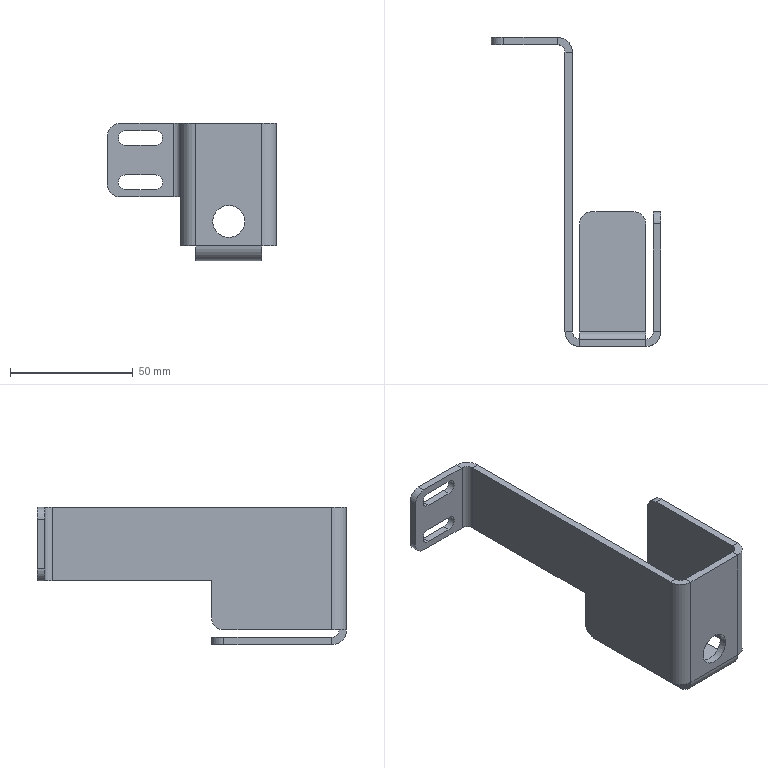Part | NX | features BREP 1 | 1 solid | 55 faces | box 69 x 126 x 56 mm | volume 33216 mm3 | plane 35 | cylinder 20 | commonest cylinder face diameters 6 x8 10 x7 12 x4 13 x1
STEP:
#1=CARTESIAN_POINT('',(0.,117.,30.));
#2=VERTEX_POINT('',#1);
#3=CARTESIAN_POINT('',(-3.,117.,30.));
#4=VERTEX_POINT('',#3);
#5=CARTESIAN_POINT('',(0.,117.,30.));
#6=DIRECTION('',(-1.,0.,0.));
#7=VECTOR('',#6,1000.);
#8=LINE('',#5,#7);
#9=EDGE_CURVE('',#2,#4,#8,.T.);
#10=ORIENTED_EDGE('',*,*,#9,.F.);
#11=CARTESIAN_POINT('',(-6.,123.,30.));
#12=VERTEX_POINT('',#11);
#13=CARTESIAN_POINT('',(-6.,117.,30.));
#14=DIRECTION('',(0.,0.,-1.));
#15=DIRECTION('',(1.,0.,0.));
#16=AXIS2_PLACEMENT_3D('',#13,#14,#15);
#17=CIRCLE('',#16,6.);
#18=EDGE_CURVE('',#12,#2,#17,.T.);
#19=ORIENTED_EDGE('',*,*,#18,.F.);
#20=CARTESIAN_POINT('',(-6.,120.,30.));
#21=VERTEX_POINT('',#20);
#22=CARTESIAN_POINT('',(-6.,120.,30.));
#23=DIRECTION('',(0.,1.,0.));
#24=VECTOR('',#23,1000.);
#25=LINE('',#22,#24);
#26=EDGE_CURVE('',#21,#12,#25,.T.);
#27=ORIENTED_EDGE('',*,*,#26,.F.);
#28=CARTESIAN_POINT('',(-6.,117.,30.));
#29=DIRECTION('',(0.,0.,-1.));
#30=DIRECTION('',(1.,0.,0.));
#31=AXIS2_PLACEMENT_3D('',#28,#29,#30);
#32=CIRCLE('',#31,3.);
#33=EDGE_CURVE('',#21,#4,#32,.T.);
#34=ORIENTED_EDGE('',*,*,#33,.T.);
#35=EDGE_LOOP('',(#10,#19,#27,#34));
#36=FACE_BOUND('',#35,.T.);
#37=CARTESIAN_POINT('',(0.,117.,30.));
#38=DIRECTION('',(0.,0.,1.));
#39=DIRECTION('',(-1.,0.,0.));
#40=AXIS2_PLACEMENT_3D('',#37,#38,#39);
#41=PLANE('',#40);
#42=ADVANCED_FACE('',(#36),#41,.T.);
#43=CARTESIAN_POINT('',(0.,3.,30.));
#44=VERTEX_POINT('',#43);
#45=CARTESIAN_POINT('',(0.,123.,30.));
#46=DIRECTION('',(0.,-1.,0.));
#47=VECTOR('',#46,1000.);
#48=LINE('',#45,#47);
#49=EDGE_CURVE('',#2,#44,#48,.T.);
#50=ORIENTED_EDGE('',*,*,#49,.F.);
#51=ORIENTED_EDGE('',*,*,#9,.T.);
#52=CARTESIAN_POINT('',(-3.,3.,30.));
#53=VERTEX_POINT('',#52);
#54=CARTESIAN_POINT('',(-3.,123.,30.));
#55=DIRECTION('',(0.,-1.,0.));
#56=VECTOR('',#55,1000.);
#57=LINE('',#54,#56);
#58=EDGE_CURVE('',#4,#53,#57,.T.);
#59=ORIENTED_EDGE('',*,*,#58,.T.);
#60=CARTESIAN_POINT('',(-3.,3.,30.));
#61=DIRECTION('',(1.,0.,0.));
#62=VECTOR('',#61,1000.);
#63=LINE('',#60,#62);
#64=EDGE_CURVE('',#53,#44,#63,.T.);
#65=ORIENTED_EDGE('',*,*,#64,.T.);
#66=EDGE_LOOP('',(#50,#51,#59,#65));
#67=FACE_BOUND('',#66,.T.);
#68=CARTESIAN_POINT('',(-6.,120.,30.));
#69=DIRECTION('',(0.,0.,1.));
#70=DIRECTION('',(-1.,0.,0.));
#71=AXIS2_PLACEMENT_3D('',#68,#69,#70);
#72=PLANE('',#71);
#73=ADVANCED_FACE('',(#67),#72,.T.);
#74=CARTESIAN_POINT('',(-6.,123.,0.));
#75=VERTEX_POINT('',#74);
#76=CARTESIAN_POINT('',(-6.,120.,0.));
#77=VERTEX_POINT('',#76);
#78=CARTESIAN_POINT('',(-6.,123.,0.));
#79=DIRECTION('',(0.,-1.,0.));
#80=VECTOR('',#79,1000.);
#81=LINE('',#78,#80);
#82=EDGE_CURVE('',#75,#77,#81,.T.);
#83=ORIENTED_EDGE('',*,*,#82,.F.);
#84=CARTESIAN_POINT('',(0.,117.,0.));
#85=VERTEX_POINT('',#84);
#86=CARTESIAN_POINT('',(-6.,117.,0.));
#87=DIRECTION('',(0.,0.,-1.));
#88=DIRECTION('',(1.,0.,0.));
#89=AXIS2_PLACEMENT_3D('',#86,#87,#88);
#90=CIRCLE('',#89,6.);
#91=EDGE_CURVE('',#75,#85,#90,.T.);
#92=ORIENTED_EDGE('',*,*,#91,.T.);
#93=CARTESIAN_POINT('',(-3.,117.,0.));
#94=VERTEX_POINT('',#93);
#95=CARTESIAN_POINT('',(-3.,117.,0.));
#96=DIRECTION('',(1.,0.,0.));
#97=VECTOR('',#96,1000.);
#98=LINE('',#95,#97);
#99=EDGE_CURVE('',#94,#85,#98,.T.);
#100=ORIENTED_EDGE('',*,*,#99,.F.);
#101=CARTESIAN_POINT('',(-6.,117.,0.));
#102=DIRECTION('',(0.,0.,-1.));
#103=DIRECTION('',(1.,0.,0.));
#104=AXIS2_PLACEMENT_3D('',#101,#102,#103);
#105=CIRCLE('',#104,3.);
#106=EDGE_CURVE('',#77,#94,#105,.T.);
#107=ORIENTED_EDGE('',*,*,#106,.F.);
#108=EDGE_LOOP('',(#83,#92,#100,#107));
#109=FACE_BOUND('',#108,.T.);
#110=CARTESIAN_POINT('',(-6.,123.,0.));
#111=DIRECTION('',(0.,0.,-1.));
#112=DIRECTION('',(1.,0.,0.));
#113=AXIS2_PLACEMENT_3D('',#110,#111,#112);
#114=PLANE('',#113);
#115=ADVANCED_FACE('',(#109),#114,.T.);
#116=CARTESIAN_POINT('',(-28.,120.,0.));
#117=VERTEX_POINT('',#116);
#118=CARTESIAN_POINT('',(-33.,120.,0.));
#119=DIRECTION('',(1.,0.,0.));
#120=VECTOR('',#119,1000.);
#121=LINE('',#118,#120);
#122=EDGE_CURVE('',#117,#77,#121,.T.);
#123=ORIENTED_EDGE('',*,*,#122,.F.);
#124=CARTESIAN_POINT('',(-28.,123.,0.));
#125=VERTEX_POINT('',#124);
#126=CARTESIAN_POINT('',(-28.,117.,0.));
#127=DIRECTION('',(0.,1.,0.));
#128=VECTOR('',#127,1000.);
#129=LINE('',#126,#128);
#130=EDGE_CURVE('',#117,#125,#129,.T.);
#131=ORIENTED_EDGE('',*,*,#130,.T.);
#132=CARTESIAN_POINT('',(-33.,123.,0.));
#133=DIRECTION('',(1.,0.,0.));
#134=VECTOR('',#133,1000.);
#135=LINE('',#132,#134);
#136=EDGE_CURVE('',#125,#75,#135,.T.);
#137=ORIENTED_EDGE('',*,*,#136,.T.);
#138=ORIENTED_EDGE('',*,*,#82,.T.);
#139=EDGE_LOOP('',(#123,#131,#137,#138));
#140=FACE_BOUND('',#139,.T.);
#141=CARTESIAN_POINT('',(-3.,117.,0.));
#142=DIRECTION('',(0.,0.,-1.));
#143=DIRECTION('',(1.,0.,0.));
#144=AXIS2_PLACEMENT_3D('',#141,#142,#143);
#145=PLANE('',#144);
#146=ADVANCED_FACE('',(#140),#145,.T.);
#147=CARTESIAN_POINT('',(3.,0.,30.));
#148=VERTEX_POINT('',#147);
#149=CARTESIAN_POINT('',(3.,-3.,30.));
#150=VERTEX_POINT('',#149);
#151=CARTESIAN_POINT('',(3.,0.,30.));
#152=DIRECTION('',(0.,-1.,0.));
#153=VECTOR('',#152,1000.);
#154=LINE('',#151,#153);
#155=EDGE_CURVE('',#148,#150,#154,.T.);
#156=ORIENTED_EDGE('',*,*,#155,.F.);
#157=CARTESIAN_POINT('',(3.,3.,30.));
#158=DIRECTION('',(0.,0.,1.));
#159=DIRECTION('',(-1.,0.,0.));
#160=AXIS2_PLACEMENT_3D('',#157,#158,#159);
#161=CIRCLE('',#160,3.);
#162=EDGE_CURVE('',#44,#148,#161,.T.);
#163=ORIENTED_EDGE('',*,*,#162,.F.);
#164=ORIENTED_EDGE('',*,*,#64,.F.);
#165=CARTESIAN_POINT('',(3.,3.,30.));
#166=DIRECTION('',(0.,0.,1.));
#167=DIRECTION('',(1.,0.,0.));
#168=AXIS2_PLACEMENT_3D('',#165,#166,#167);
#169=CIRCLE('',#168,6.);
#170=EDGE_CURVE('',#53,#150,#169,.T.);
#171=ORIENTED_EDGE('',*,*,#170,.T.);
#172=EDGE_LOOP('',(#156,#163,#164,#171));
#173=FACE_BOUND('',#172,.T.);
#174=CARTESIAN_POINT('',(3.,0.,30.));
#175=DIRECTION('',(0.,0.,1.));
#176=DIRECTION('',(-1.,0.,0.));
#177=AXIS2_PLACEMENT_3D('',#174,#175,#176);
#178=PLANE('',#177);
#179=ADVANCED_FACE('',(#173),#178,.T.);
#180=CARTESIAN_POINT('',(30.,0.,30.));
#181=VERTEX_POINT('',#180);
#182=CARTESIAN_POINT('',(0.,0.,30.));
#183=DIRECTION('',(1.,0.,0.));
#184=VECTOR('',#183,1000.);
#185=LINE('',#182,#184);
#186=EDGE_CURVE('',#148,#181,#185,.T.);
#187=ORIENTED_EDGE('',*,*,#186,.F.);
#188=ORIENTED_EDGE('',*,*,#155,.T.);
#189=CARTESIAN_POINT('',(30.,-3.,30.));
#190=VERTEX_POINT('',#189);
#191=CARTESIAN_POINT('',(0.,-3.,30.));
#192=DIRECTION('',(1.,0.,0.));
#193=VECTOR('',#192,1000.);
#194=LINE('',#191,#193);
#195=EDGE_CURVE('',#150,#190,#194,.T.);
#196=ORIENTED_EDGE('',*,*,#195,.T.);
#197=CARTESIAN_POINT('',(30.,0.,30.));
#198=DIRECTION('',(0.,-1.,0.));
#199=VECTOR('',#198,1000.);
#200=LINE('',#197,#199);
#201=EDGE_CURVE('',#181,#190,#200,.T.);
#202=ORIENTED_EDGE('',*,*,#201,.F.);
#203=EDGE_LOOP('',(#187,#188,#196,#202));
#204=FACE_BOUND('',#203,.T.);
#205=CARTESIAN_POINT('',(-3.,3.,30.));
#206=DIRECTION('',(0.,0.,1.));
#207=DIRECTION('',(-1.,0.,0.));
#208=AXIS2_PLACEMENT_3D('',#205,#206,#207);
#209=PLANE('',#208);
#210=ADVANCED_FACE('',(#204),#209,.T.);
#211=CARTESIAN_POINT('',(0.,52.,0.));
#212=VERTEX_POINT('',#211);
#213=CARTESIAN_POINT('',(0.,123.,0.));
#214=DIRECTION('',(0.,-1.,0.));
#215=VECTOR('',#214,1000.);
#216=LINE('',#213,#215);
#217=EDGE_CURVE('',#85,#212,#216,.T.);
#218=ORIENTED_EDGE('',*,*,#217,.T.);
#219=CARTESIAN_POINT('',(-3.,52.,0.));
#220=VERTEX_POINT('',#219);
#221=CARTESIAN_POINT('',(-3.,52.,0.));
#222=DIRECTION('',(1.,0.,0.));
#223=VECTOR('',#222,1000.);
#224=LINE('',#221,#223);
#225=EDGE_CURVE('',#220,#212,#224,.T.);
#226=ORIENTED_EDGE('',*,*,#225,.F.);
#227=CARTESIAN_POINT('',(-3.,123.,0.));
#228=DIRECTION('',(0.,-1.,0.));
#229=VECTOR('',#228,1000.);
#230=LINE('',#227,#229);
#231=EDGE_CURVE('',#94,#220,#230,.T.);
#232=ORIENTED_EDGE('',*,*,#231,.F.);
#233=ORIENTED_EDGE('',*,*,#99,.T.);
#234=EDGE_LOOP('',(#218,#226,#232,#233));
#235=FACE_BOUND('',#234,.T.);
#236=CARTESIAN_POINT('',(3.,-3.,0.));
#237=DIRECTION('',(0.,0.,-1.));
#238=DIRECTION('',(1.,0.,0.));
#239=AXIS2_PLACEMENT_3D('',#236,#237,#238);
#240=PLANE('',#239);
#241=ADVANCED_FACE('',(#235),#240,.T.);
#242=CARTESIAN_POINT('',(16.5,-3.,-16.5));
#243=VERTEX_POINT('',#242);
#244=CARTESIAN_POINT('',(16.5,-3.,-10.));
#245=DIRECTION('',(0.,-1.,0.));
#246=DIRECTION('',(0.,0.,-1.));
#247=AXIS2_PLACEMENT_3D('',#244,#245,#246);
#248=CIRCLE('',#247,6.5);
#249=EDGE_CURVE('',#243,#243,#248,.T.);
#250=ORIENTED_EDGE('',*,*,#249,.F.);
#251=EDGE_LOOP('',(#250));
#252=FACE_BOUND('',#251,.T.);
#253=CARTESIAN_POINT('',(3.,-3.,-20.));
#254=VERTEX_POINT('',#253);
#255=CARTESIAN_POINT('',(3.,-3.,30.));
#256=DIRECTION('',(0.,0.,-1.));
#257=VECTOR('',#256,1000.);
#258=LINE('',#255,#257);
#259=EDGE_CURVE('',#150,#254,#258,.T.);
#260=ORIENTED_EDGE('',*,*,#259,.T.);
#261=CARTESIAN_POINT('',(30.,-3.,-20.));
#262=VERTEX_POINT('',#261);
#263=CARTESIAN_POINT('',(3.,-3.,-20.));
#264=DIRECTION('',(1.,0.,0.));
#265=VECTOR('',#264,1000.);
#266=LINE('',#263,#265);
#267=EDGE_CURVE('',#254,#262,#266,.T.);
#268=ORIENTED_EDGE('',*,*,#267,.T.);
#269=CARTESIAN_POINT('',(30.,-3.,30.));
#270=DIRECTION('',(0.,0.,-1.));
#271=VECTOR('',#270,1000.);
#272=LINE('',#269,#271);
#273=EDGE_CURVE('',#190,#262,#272,.T.);
#274=ORIENTED_EDGE('',*,*,#273,.F.);
#275=ORIENTED_EDGE('',*,*,#195,.F.);
#276=EDGE_LOOP('',(#260,#268,#274,#275));
#277=FACE_BOUND('',#276,.T.);
#278=CARTESIAN_POINT('',(0.,-3.,30.));
#279=DIRECTION('',(0.,1.,0.));
#280=DIRECTION('',(0.,0.,-1.));
#281=AXIS2_PLACEMENT_3D('',#278,#279,#280);
#282=PLANE('',#281);
#283=ADVANCED_FACE('',(#252,#277),#282,.F.);
#284=CARTESIAN_POINT('',(16.5,0.,-3.5));
#285=VERTEX_POINT('',#284);
#286=CARTESIAN_POINT('',(16.5,0.,-10.));
#287=DIRECTION('',(0.,1.,0.));
#288=DIRECTION('',(0.,0.,1.));
#289=AXIS2_PLACEMENT_3D('',#286,#287,#288);
#290=CIRCLE('',#289,6.5);
#291=EDGE_CURVE('',#285,#285,#290,.T.);
#292=ORIENTED_EDGE('',*,*,#291,.F.);
#293=EDGE_LOOP('',(#292));
#294=FACE_BOUND('',#293,.T.);
#295=CARTESIAN_POINT('',(30.,0.,-20.));
#296=VERTEX_POINT('',#295);
#297=CARTESIAN_POINT('',(30.,0.,30.));
#298=DIRECTION('',(0.,0.,-1.));
#299=VECTOR('',#298,1000.);
#300=LINE('',#297,#299);
#301=EDGE_CURVE('',#181,#296,#300,.T.);
#302=ORIENTED_EDGE('',*,*,#301,.T.);
#303=CARTESIAN_POINT('',(3.,0.,-20.));
#304=VERTEX_POINT('',#303);
#305=CARTESIAN_POINT('',(3.,0.,-20.));
#306=DIRECTION('',(1.,0.,0.));
#307=VECTOR('',#306,1000.);
#308=LINE('',#305,#307);
#309=EDGE_CURVE('',#304,#296,#308,.T.);
#310=ORIENTED_EDGE('',*,*,#309,.F.);
#311=CARTESIAN_POINT('',(3.,0.,30.));
#312=DIRECTION('',(0.,0.,-1.));
#313=VECTOR('',#312,1000.);
#314=LINE('',#311,#313);
#315=EDGE_CURVE('',#148,#304,#314,.T.);
#316=ORIENTED_EDGE('',*,*,#315,.F.);
#317=ORIENTED_EDGE('',*,*,#186,.T.);
#318=EDGE_LOOP('',(#302,#310,#316,#317));
#319=FACE_BOUND('',#318,.T.);
#320=CARTESIAN_POINT('',(0.,0.,30.));
#321=DIRECTION('',(0.,1.,0.));
#322=DIRECTION('',(0.,0.,-1.));
#323=AXIS2_PLACEMENT_3D('',#320,#321,#322);
#324=PLANE('',#323);
#325=ADVANCED_FACE('',(#294,#319),#324,.T.);
#326=ORIENTED_EDGE('',*,*,#315,.T.);
#327=CARTESIAN_POINT('',(0.,3.,-20.));
#328=VERTEX_POINT('',#327);
#329=CARTESIAN_POINT('',(3.,3.,-20.));
#330=DIRECTION('',(0.,0.,1.));
#331=DIRECTION('',(1.,0.,0.));
#332=AXIS2_PLACEMENT_3D('',#329,#330,#331);
#333=CIRCLE('',#332,3.);
#334=EDGE_CURVE('',#328,#304,#333,.T.);
#335=ORIENTED_EDGE('',*,*,#334,.F.);
#336=CARTESIAN_POINT('',(0.,3.,30.));
#337=DIRECTION('',(0.,0.,-1.));
#338=VECTOR('',#337,1000.);
#339=LINE('',#336,#338);
#340=EDGE_CURVE('',#44,#328,#339,.T.);
#341=ORIENTED_EDGE('',*,*,#340,.F.);
#342=ORIENTED_EDGE('',*,*,#162,.T.);
#343=EDGE_LOOP('',(#326,#335,#341,#342));
#344=FACE_BOUND('',#343,.T.);
#345=CARTESIAN_POINT('',(3.,3.,30.));
#346=DIRECTION('',(0.,0.,-1.));
#347=DIRECTION('',(1.,0.,0.));
#348=AXIS2_PLACEMENT_3D('',#345,#346,#347);
#349=CYLINDRICAL_SURFACE('',#348,3.);
#350=ADVANCED_FACE('',(#344),#349,.F.);
#351=CARTESIAN_POINT('',(0.,47.,-20.));
#352=VERTEX_POINT('',#351);
#353=CARTESIAN_POINT('',(0.,52.,-20.));
#354=DIRECTION('',(0.,-1.,0.));
#355=VECTOR('',#354,1000.);
#356=LINE('',#353,#355);
#357=EDGE_CURVE('',#352,#328,#356,.T.);
#358=ORIENTED_EDGE('',*,*,#357,.F.);
#359=CARTESIAN_POINT('',(0.,52.,-15.));
#360=VERTEX_POINT('',#359);
#361=CARTESIAN_POINT('',(0.,47.,-15.));
#362=DIRECTION('',(1.,0.,0.));
#363=DIRECTION('',(0.,1.,0.));
#364=AXIS2_PLACEMENT_3D('',#361,#362,#363);
#365=CIRCLE('',#364,5.);
#366=EDGE_CURVE('',#352,#360,#365,.T.);
#367=ORIENTED_EDGE('',*,*,#366,.T.);
#368=CARTESIAN_POINT('',(0.,52.,-20.));
#369=DIRECTION('',(0.,0.,1.));
#370=VECTOR('',#369,1000.);
#371=LINE('',#368,#370);
#372=EDGE_CURVE('',#360,#212,#371,.T.);
#373=ORIENTED_EDGE('',*,*,#372,.T.);
#374=ORIENTED_EDGE('',*,*,#217,.F.);
#375=CARTESIAN_POINT('',(0.,117.,30.));
#376=DIRECTION('',(0.,0.,-1.));
#377=VECTOR('',#376,1000.);
#378=LINE('',#375,#377);
#379=EDGE_CURVE('',#2,#85,#378,.T.);
#380=ORIENTED_EDGE('',*,*,#379,.F.);
#381=ORIENTED_EDGE('',*,*,#49,.T.);
#382=ORIENTED_EDGE('',*,*,#340,.T.);
#383=EDGE_LOOP('',(#358,#367,#373,#374,#380,#381,#382));
#384=FACE_BOUND('',#383,.T.);
#385=CARTESIAN_POINT('',(0.,123.,30.));
#386=DIRECTION('',(1.,0.,0.));
#387=DIRECTION('',(0.,-1.,0.));
#388=AXIS2_PLACEMENT_3D('',#385,#386,#387);
#389=PLANE('',#388);
#390=ADVANCED_FACE('',(#384),#389,.T.);
#391=ORIENTED_EDGE('',*,*,#91,.F.);
#392=CARTESIAN_POINT('',(-6.,123.,30.));
#393=DIRECTION('',(0.,0.,-1.));
#394=VECTOR('',#393,1000.);
#395=LINE('',#392,#394);
#396=EDGE_CURVE('',#12,#75,#395,.T.);
#397=ORIENTED_EDGE('',*,*,#396,.F.);
#398=ORIENTED_EDGE('',*,*,#18,.T.);
#399=ORIENTED_EDGE('',*,*,#379,.T.);
#400=EDGE_LOOP('',(#391,#397,#398,#399));
#401=FACE_BOUND('',#400,.T.);
#402=CARTESIAN_POINT('',(-6.,117.,30.));
#403=DIRECTION('',(0.,0.,-1.));
#404=DIRECTION('',(1.,0.,0.));
#405=AXIS2_PLACEMENT_3D('',#402,#403,#404);
#406=CYLINDRICAL_SURFACE('',#405,6.);
#407=ADVANCED_FACE('',(#401),#406,.T.);
#408=CARTESIAN_POINT('',(-25.5,123.,21.));
#409=VERTEX_POINT('',#408);
#410=CARTESIAN_POINT('',(-25.5,123.,27.));
#411=VERTEX_POINT('',#410);
#412=CARTESIAN_POINT('',(-25.5,123.,24.));
#413=DIRECTION('',(0.,1.,0.));
#414=DIRECTION('',(0.,0.,1.));
#415=AXIS2_PLACEMENT_3D('',#412,#413,#414);
#416=CIRCLE('',#415,3.);
#417=EDGE_CURVE('',#409,#411,#416,.T.);
#418=ORIENTED_EDGE('',*,*,#417,.F.);
#419=CARTESIAN_POINT('',(-13.5,123.,21.));
#420=VERTEX_POINT('',#419);
#421=CARTESIAN_POINT('',(-25.5,123.,21.));
#422=DIRECTION('',(-1.,0.,0.));
#423=VECTOR('',#422,1000.);
#424=LINE('',#421,#423);
#425=EDGE_CURVE('',#420,#409,#424,.T.);
#426=ORIENTED_EDGE('',*,*,#425,.F.);
#427=CARTESIAN_POINT('',(-13.5,123.,27.));
#428=VERTEX_POINT('',#427);
#429=CARTESIAN_POINT('',(-13.5,123.,24.));
#430=DIRECTION('',(0.,1.,0.));
#431=DIRECTION('',(0.,0.,1.));
#432=AXIS2_PLACEMENT_3D('',#429,#430,#431);
#433=CIRCLE('',#432,3.);
#434=EDGE_CURVE('',#428,#420,#433,.T.);
#435=ORIENTED_EDGE('',*,*,#434,.F.);
#436=CARTESIAN_POINT('',(-25.5,123.,27.));
#437=DIRECTION('',(1.,0.,0.));
#438=VECTOR('',#437,1000.);
#439=LINE('',#436,#438);
#440=EDGE_CURVE('',#411,#428,#439,.T.);
#441=ORIENTED_EDGE('',*,*,#440,.F.);
#442=EDGE_LOOP('',(#418,#426,#435,#441));
#443=FACE_BOUND('',#442,.T.);
#444=CARTESIAN_POINT('',(-25.5,123.,3.));
#445=VERTEX_POINT('',#444);
#446=CARTESIAN_POINT('',(-25.5,123.,9.));
#447=VERTEX_POINT('',#446);
#448=CARTESIAN_POINT('',(-25.5,123.,6.));
#449=DIRECTION('',(0.,1.,0.));
#450=DIRECTION('',(0.,0.,1.));
#451=AXIS2_PLACEMENT_3D('',#448,#449,#450);
#452=CIRCLE('',#451,3.);
#453=EDGE_CURVE('',#445,#447,#452,.T.);
#454=ORIENTED_EDGE('',*,*,#453,.F.);
#455=CARTESIAN_POINT('',(-13.5,123.,3.));
#456=VERTEX_POINT('',#455);
#457=CARTESIAN_POINT('',(-25.5,123.,3.));
#458=DIRECTION('',(-1.,0.,0.));
#459=VECTOR('',#458,1000.);
#460=LINE('',#457,#459);
#461=EDGE_CURVE('',#456,#445,#460,.T.);
#462=ORIENTED_EDGE('',*,*,#461,.F.);
#463=CARTESIAN_POINT('',(-13.5,123.,9.));
#464=VERTEX_POINT('',#463);
#465=CARTESIAN_POINT('',(-13.5,123.,6.));
#466=DIRECTION('',(0.,1.,0.));
#467=DIRECTION('',(0.,0.,1.));
#468=AXIS2_PLACEMENT_3D('',#465,#466,#467);
#469=CIRCLE('',#468,3.);
#470=EDGE_CURVE('',#464,#456,#469,.T.);
#471=ORIENTED_EDGE('',*,*,#470,.F.);
#472=CARTESIAN_POINT('',(-25.5,123.,9.));
#473=DIRECTION('',(1.,0.,0.));
#474=VECTOR('',#473,1000.);
#475=LINE('',#472,#474);
#476=EDGE_CURVE('',#447,#464,#475,.T.);
#477=ORIENTED_EDGE('',*,*,#476,.F.);
#478=EDGE_LOOP('',(#454,#462,#471,#477));
#479=FACE_BOUND('',#478,.T.);
#480=ORIENTED_EDGE('',*,*,#136,.F.);
#481=CARTESIAN_POINT('',(-33.,123.,5.));
#482=VERTEX_POINT('',#481);
#483=CARTESIAN_POINT('',(-28.,123.,5.));
#484=DIRECTION('',(0.,1.,0.));
#485=DIRECTION('',(0.,0.,1.));
#486=AXIS2_PLACEMENT_3D('',#483,#484,#485);
#487=CIRCLE('',#486,5.);
#488=EDGE_CURVE('',#125,#482,#487,.T.);
#489=ORIENTED_EDGE('',*,*,#488,.T.);
#490=CARTESIAN_POINT('',(-33.,123.,25.));
#491=VERTEX_POINT('',#490);
#492=CARTESIAN_POINT('',(-33.,123.,30.));
#493=DIRECTION('',(0.,0.,-1.));
#494=VECTOR('',#493,1000.);
#495=LINE('',#492,#494);
#496=EDGE_CURVE('',#491,#482,#495,.T.);
#497=ORIENTED_EDGE('',*,*,#496,.F.);
#498=CARTESIAN_POINT('',(-28.,123.,30.));
#499=VERTEX_POINT('',#498);
#500=CARTESIAN_POINT('',(-28.,123.,25.));
#501=DIRECTION('',(0.,1.,0.));
#502=DIRECTION('',(0.,0.,1.));
#503=AXIS2_PLACEMENT_3D('',#500,#501,#502);
#504=CIRCLE('',#503,5.);
#505=EDGE_CURVE('',#491,#499,#504,.T.);
#506=ORIENTED_EDGE('',*,*,#505,.T.);
#507=CARTESIAN_POINT('',(-33.,123.,30.));
#508=DIRECTION('',(1.,0.,0.));
#509=VECTOR('',#508,1000.);
#510=LINE('',#507,#509);
#511=EDGE_CURVE('',#499,#12,#510,.T.);
#512=ORIENTED_EDGE('',*,*,#511,.T.);
#513=ORIENTED_EDGE('',*,*,#396,.T.);
#514=EDGE_LOOP('',(#480,#489,#497,#506,#512,#513));
#515=FACE_BOUND('',#514,.T.);
#516=CARTESIAN_POINT('',(-33.,123.,30.));
#517=DIRECTION('',(0.,1.,0.));
#518=DIRECTION('',(0.,0.,-1.));
#519=AXIS2_PLACEMENT_3D('',#516,#517,#518);
#520=PLANE('',#519);
#521=ADVANCED_FACE('',(#443,#479,#515),#520,.T.);
#522=ORIENTED_EDGE('',*,*,#496,.T.);
#523=CARTESIAN_POINT('',(-33.,120.,5.));
#524=VERTEX_POINT('',#523);
#525=CARTESIAN_POINT('',(-33.,120.,5.));
#526=DIRECTION('',(0.,-1.,0.));
#527=VECTOR('',#526,1000.);
#528=LINE('',#525,#527);
#529=EDGE_CURVE('',#482,#524,#528,.T.);
#530=ORIENTED_EDGE('',*,*,#529,.T.);
#531=CARTESIAN_POINT('',(-33.,120.,25.));
#532=VERTEX_POINT('',#531);
#533=CARTESIAN_POINT('',(-33.,120.,30.));
#534=DIRECTION('',(0.,0.,-1.));
#535=VECTOR('',#534,1000.);
#536=LINE('',#533,#535);
#537=EDGE_CURVE('',#532,#524,#536,.T.);
#538=ORIENTED_EDGE('',*,*,#537,.F.);
#539=CARTESIAN_POINT('',(-33.,123.,25.));
#540=DIRECTION('',(0.,1.,0.));
#541=VECTOR('',#540,1000.);
#542=LINE('',#539,#541);
#543=EDGE_CURVE('',#532,#491,#542,.T.);
#544=ORIENTED_EDGE('',*,*,#543,.T.);
#545=EDGE_LOOP('',(#522,#530,#538,#544));
#546=FACE_BOUND('',#545,.T.);
#547=CARTESIAN_POINT('',(-33.,120.,30.));
#548=DIRECTION('',(-1.,0.,0.));
#549=DIRECTION('',(0.,0.,-1.));
#550=AXIS2_PLACEMENT_3D('',#547,#548,#549);
#551=PLANE('',#550);
#552=ADVANCED_FACE('',(#546),#551,.T.);
#553=CARTESIAN_POINT('',(-13.5,120.,21.));
#554=VERTEX_POINT('',#553);
#555=CARTESIAN_POINT('',(-25.5,120.,21.));
#556=VERTEX_POINT('',#555);
#557=CARTESIAN_POINT('',(-33.,120.,21.));
#558=DIRECTION('',(-1.,0.,0.));
#559=VECTOR('',#558,1000.);
#560=LINE('',#557,#559);
#561=EDGE_CURVE('',#554,#556,#560,.T.);
#562=ORIENTED_EDGE('',*,*,#561,.T.);
#563=CARTESIAN_POINT('',(-25.5,120.,27.));
#564=VERTEX_POINT('',#563);
#565=CARTESIAN_POINT('',(-25.5,120.,24.));
#566=DIRECTION('',(0.,1.,0.));
#567=DIRECTION('',(0.,0.,1.));
#568=AXIS2_PLACEMENT_3D('',#565,#566,#567);
#569=CIRCLE('',#568,3.);
#570=EDGE_CURVE('',#556,#564,#569,.T.);
#571=ORIENTED_EDGE('',*,*,#570,.T.);
#572=CARTESIAN_POINT('',(-13.5,120.,27.));
#573=VERTEX_POINT('',#572);
#574=CARTESIAN_POINT('',(-33.,120.,27.));
#575=DIRECTION('',(1.,0.,0.));
#576=VECTOR('',#575,1000.);
#577=LINE('',#574,#576);
#578=EDGE_CURVE('',#564,#573,#577,.T.);
#579=ORIENTED_EDGE('',*,*,#578,.T.);
#580=CARTESIAN_POINT('',(-13.5,120.,24.));
#581=DIRECTION('',(0.,1.,0.));
#582=DIRECTION('',(0.,0.,1.));
#583=AXIS2_PLACEMENT_3D('',#580,#581,#582);
#584=CIRCLE('',#583,3.);
#585=EDGE_CURVE('',#573,#554,#584,.T.);
#586=ORIENTED_EDGE('',*,*,#585,.T.);
#587=EDGE_LOOP('',(#562,#571,#579,#586));
#588=FACE_BOUND('',#587,.T.);
#589=CARTESIAN_POINT('',(-13.5,120.,3.));
#590=VERTEX_POINT('',#589);
#591=CARTESIAN_POINT('',(-25.5,120.,3.));
#592=VERTEX_POINT('',#591);
#593=CARTESIAN_POINT('',(-33.,120.,3.));
#594=DIRECTION('',(-1.,0.,0.));
#595=VECTOR('',#594,1000.);
#596=LINE('',#593,#595);
#597=EDGE_CURVE('',#590,#592,#596,.T.);
#598=ORIENTED_EDGE('',*,*,#597,.T.);
#599=CARTESIAN_POINT('',(-25.5,120.,9.));
#600=VERTEX_POINT('',#599);
#601=CARTESIAN_POINT('',(-25.5,120.,6.));
#602=DIRECTION('',(0.,1.,0.));
#603=DIRECTION('',(0.,0.,1.));
#604=AXIS2_PLACEMENT_3D('',#601,#602,#603);
#605=CIRCLE('',#604,3.);
#606=EDGE_CURVE('',#592,#600,#605,.T.);
#607=ORIENTED_EDGE('',*,*,#606,.T.);
#608=CARTESIAN_POINT('',(-13.5,120.,9.));
#609=VERTEX_POINT('',#608);
#610=CARTESIAN_POINT('',(-33.,120.,9.));
#611=DIRECTION('',(1.,0.,0.));
#612=VECTOR('',#611,1000.);
#613=LINE('',#610,#612);
#614=EDGE_CURVE('',#600,#609,#613,.T.);
#615=ORIENTED_EDGE('',*,*,#614,.T.);
#616=CARTESIAN_POINT('',(-13.5,120.,6.));
#617=DIRECTION('',(0.,1.,0.));
#618=DIRECTION('',(0.,0.,1.));
#619=AXIS2_PLACEMENT_3D('',#616,#617,#618);
#620=CIRCLE('',#619,3.);
#621=EDGE_CURVE('',#609,#590,#620,.T.);
#622=ORIENTED_EDGE('',*,*,#621,.T.);
#623=EDGE_LOOP('',(#598,#607,#615,#622));
#624=FACE_BOUND('',#623,.T.);
#625=ORIENTED_EDGE('',*,*,#537,.T.);
#626=CARTESIAN_POINT('',(-28.,120.,5.));
#627=DIRECTION('',(0.,-1.,0.));
#628=DIRECTION('',(0.,0.,1.));
#629=AXIS2_PLACEMENT_3D('',#626,#627,#628);
#630=CIRCLE('',#629,5.);
#631=EDGE_CURVE('',#524,#117,#630,.T.);
#632=ORIENTED_EDGE('',*,*,#631,.T.);
#633=ORIENTED_EDGE('',*,*,#122,.T.);
#634=CARTESIAN_POINT('',(-6.,120.,30.));
#635=DIRECTION('',(0.,0.,-1.));
#636=VECTOR('',#635,1000.);
#637=LINE('',#634,#636);
#638=EDGE_CURVE('',#21,#77,#637,.T.);
#639=ORIENTED_EDGE('',*,*,#638,.F.);
#640=CARTESIAN_POINT('',(-28.,120.,30.));
#641=VERTEX_POINT('',#640);
#642=CARTESIAN_POINT('',(-33.,120.,30.));
#643=DIRECTION('',(1.,0.,0.));
#644=VECTOR('',#643,1000.);
#645=LINE('',#642,#644);
#646=EDGE_CURVE('',#641,#21,#645,.T.);
#647=ORIENTED_EDGE('',*,*,#646,.F.);
#648=CARTESIAN_POINT('',(-28.,120.,25.));
#649=DIRECTION('',(0.,-1.,0.));
#650=DIRECTION('',(0.,0.,1.));
#651=AXIS2_PLACEMENT_3D('',#648,#649,#650);
#652=CIRCLE('',#651,5.);
#653=EDGE_CURVE('',#641,#532,#652,.T.);
#654=ORIENTED_EDGE('',*,*,#653,.T.);
#655=EDGE_LOOP('',(#625,#632,#633,#639,#647,#654));
#656=FACE_BOUND('',#655,.T.);
#657=CARTESIAN_POINT('',(-33.,120.,30.));
#658=DIRECTION('',(0.,1.,0.));
#659=DIRECTION('',(0.,0.,-1.));
#660=AXIS2_PLACEMENT_3D('',#657,#658,#659);
#661=PLANE('',#660);
#662=ADVANCED_FACE('',(#588,#624,#656),#661,.F.);
#663=ORIENTED_EDGE('',*,*,#106,.T.);
#664=CARTESIAN_POINT('',(-3.,117.,30.));
#665=DIRECTION('',(0.,0.,-1.));
#666=VECTOR('',#665,1000.);
#667=LINE('',#664,#666);
#668=EDGE_CURVE('',#4,#94,#667,.T.);
#669=ORIENTED_EDGE('',*,*,#668,.F.);
#670=ORIENTED_EDGE('',*,*,#33,.F.);
#671=ORIENTED_EDGE('',*,*,#638,.T.);
#672=EDGE_LOOP('',(#663,#669,#670,#671));
#673=FACE_BOUND('',#672,.T.);
#674=CARTESIAN_POINT('',(-6.,117.,30.));
#675=DIRECTION('',(0.,0.,-1.));
#676=DIRECTION('',(1.,0.,0.));
#677=AXIS2_PLACEMENT_3D('',#674,#675,#676);
#678=CYLINDRICAL_SURFACE('',#677,3.);
#679=ADVANCED_FACE('',(#673),#678,.F.);
#680=CARTESIAN_POINT('',(-3.,52.,-15.));
#681=VERTEX_POINT('',#680);
#682=CARTESIAN_POINT('',(-3.,52.,-20.));
#683=DIRECTION('',(0.,0.,1.));
#684=VECTOR('',#683,1000.);
#685=LINE('',#682,#684);
#686=EDGE_CURVE('',#681,#220,#685,.T.);
#687=ORIENTED_EDGE('',*,*,#686,.F.);
#688=CARTESIAN_POINT('',(-3.,47.,-20.));
#689=VERTEX_POINT('',#688);
#690=CARTESIAN_POINT('',(-3.,47.,-15.));
#691=DIRECTION('',(-1.,0.,0.));
#692=DIRECTION('',(0.,1.,0.));
#693=AXIS2_PLACEMENT_3D('',#690,#691,#692);
#694=CIRCLE('',#693,5.);
#695=EDGE_CURVE('',#681,#689,#694,.T.);
#696=ORIENTED_EDGE('',*,*,#695,.T.);
#697=CARTESIAN_POINT('',(-3.,3.,-20.));
#698=VERTEX_POINT('',#697);
#699=CARTESIAN_POINT('',(-3.,3.,-20.));
#700=DIRECTION('',(0.,1.,0.));
#701=VECTOR('',#700,1000.);
#702=LINE('',#699,#701);
#703=EDGE_CURVE('',#698,#689,#702,.T.);
#704=ORIENTED_EDGE('',*,*,#703,.F.);
#705=CARTESIAN_POINT('',(-3.,3.,30.));
#706=DIRECTION('',(0.,0.,-1.));
#707=VECTOR('',#706,1000.);
#708=LINE('',#705,#707);
#709=EDGE_CURVE('',#53,#698,#708,.T.);
#710=ORIENTED_EDGE('',*,*,#709,.F.);
#711=ORIENTED_EDGE('',*,*,#58,.F.);
#712=ORIENTED_EDGE('',*,*,#668,.T.);
#713=ORIENTED_EDGE('',*,*,#231,.T.);
#714=EDGE_LOOP('',(#687,#696,#704,#710,#711,#712,#713));
#715=FACE_BOUND('',#714,.T.);
#716=CARTESIAN_POINT('',(-3.,123.,30.));
#717=DIRECTION('',(1.,0.,0.));
#718=DIRECTION('',(0.,-1.,0.));
#719=AXIS2_PLACEMENT_3D('',#716,#717,#718);
#720=PLANE('',#719);
#721=ADVANCED_FACE('',(#715),#720,.F.);
#722=ORIENTED_EDGE('',*,*,#709,.T.);
#723=CARTESIAN_POINT('',(3.,3.,-20.));
#724=DIRECTION('',(0.,0.,-1.));
#725=DIRECTION('',(-1.,0.,0.));
#726=AXIS2_PLACEMENT_3D('',#723,#724,#725);
#727=CIRCLE('',#726,6.);
#728=EDGE_CURVE('',#254,#698,#727,.T.);
#729=ORIENTED_EDGE('',*,*,#728,.F.);
#730=ORIENTED_EDGE('',*,*,#259,.F.);
#731=ORIENTED_EDGE('',*,*,#170,.F.);
#732=EDGE_LOOP('',(#722,#729,#730,#731));
#733=FACE_BOUND('',#732,.T.);
#734=CARTESIAN_POINT('',(3.,3.,30.));
#735=DIRECTION('',(0.,0.,-1.));
#736=DIRECTION('',(1.,0.,0.));
#737=AXIS2_PLACEMENT_3D('',#734,#735,#736);
#738=CYLINDRICAL_SURFACE('',#737,6.);
#739=ADVANCED_FACE('',(#733),#738,.T.);
#740=ORIENTED_EDGE('',*,*,#511,.F.);
#741=CARTESIAN_POINT('',(-28.,120.,30.));
#742=DIRECTION('',(0.,-1.,0.));
#743=VECTOR('',#742,1000.);
#744=LINE('',#741,#743);
#745=EDGE_CURVE('',#499,#641,#744,.T.);
#746=ORIENTED_EDGE('',*,*,#745,.T.);
#747=ORIENTED_EDGE('',*,*,#646,.T.);
#748=ORIENTED_EDGE('',*,*,#26,.T.);
#749=EDGE_LOOP('',(#740,#746,#747,#748));
#750=FACE_BOUND('',#749,.T.);
#751=CARTESIAN_POINT('',(3.,3.,30.));
#752=DIRECTION('',(0.,0.,-1.));
#753=DIRECTION('',(1.,0.,0.));
#754=AXIS2_PLACEMENT_3D('',#751,#752,#753);
#755=PLANE('',#754);
#756=ADVANCED_FACE('',(#750),#755,.F.);
#757=ORIENTED_EDGE('',*,*,#703,.T.);
#758=CARTESIAN_POINT('',(0.,47.,-20.));
#759=DIRECTION('',(1.,0.,0.));
#760=VECTOR('',#759,1000.);
#761=LINE('',#758,#760);
#762=EDGE_CURVE('',#689,#352,#761,.T.);
#763=ORIENTED_EDGE('',*,*,#762,.T.);
#764=ORIENTED_EDGE('',*,*,#357,.T.);
#765=ORIENTED_EDGE('',*,*,#334,.T.);
#766=CARTESIAN_POINT('',(3.,0.,-20.));
#767=DIRECTION('',(0.,-1.,0.));
#768=VECTOR('',#767,1000.);
#769=LINE('',#766,#768);
#770=EDGE_CURVE('',#304,#254,#769,.T.);
#771=ORIENTED_EDGE('',*,*,#770,.T.);
#772=ORIENTED_EDGE('',*,*,#728,.T.);
#773=EDGE_LOOP('',(#757,#763,#764,#765,#771,#772));
#774=FACE_BOUND('',#773,.T.);
#775=CARTESIAN_POINT('',(3.,33.601,-20.));
#776=DIRECTION('',(0.,0.,-1.));
#777=DIRECTION('',(1.,0.,0.));
#778=AXIS2_PLACEMENT_3D('',#775,#776,#777);
#779=PLANE('',#778);
#780=ADVANCED_FACE('',(#774),#779,.T.);
#781=ORIENTED_EDGE('',*,*,#291,.T.);
#782=EDGE_LOOP('',(#781));
#783=FACE_BOUND('',#782,.T.);
#784=ORIENTED_EDGE('',*,*,#249,.T.);
#785=EDGE_LOOP('',(#784));
#786=FACE_BOUND('',#785,.T.);
#787=CARTESIAN_POINT('',(16.5,-3.,-10.));
#788=DIRECTION('',(0.,-1.,0.));
#789=DIRECTION('',(0.,0.,1.));
#790=AXIS2_PLACEMENT_3D('',#787,#788,#789);
#791=CYLINDRICAL_SURFACE('',#790,6.5);
#792=ADVANCED_FACE('',(#783,#786),#791,.F.);
#793=CARTESIAN_POINT('',(-25.5,113.,3.));
#794=DIRECTION('',(0.,1.,0.));
#795=VECTOR('',#794,1000.);
#796=LINE('',#793,#795);
#797=EDGE_CURVE('',#592,#445,#796,.T.);
#798=ORIENTED_EDGE('',*,*,#797,.T.);
#799=ORIENTED_EDGE('',*,*,#453,.T.);
#800=CARTESIAN_POINT('',(-25.5,113.,9.));
#801=DIRECTION('',(0.,1.,0.));
#802=VECTOR('',#801,1000.);
#803=LINE('',#800,#802);
#804=EDGE_CURVE('',#600,#447,#803,.T.);
#805=ORIENTED_EDGE('',*,*,#804,.F.);
#806=ORIENTED_EDGE('',*,*,#606,.F.);
#807=EDGE_LOOP('',(#798,#799,#805,#806));
#808=FACE_BOUND('',#807,.T.);
#809=CARTESIAN_POINT('',(-25.5,113.,6.));
#810=DIRECTION('',(0.,1.,0.));
#811=DIRECTION('',(0.,0.,-1.));
#812=AXIS2_PLACEMENT_3D('',#809,#810,#811);
#813=CYLINDRICAL_SURFACE('',#812,3.);
#814=ADVANCED_FACE('',(#808),#813,.F.);
#815=CARTESIAN_POINT('',(-13.5,113.,3.));
#816=DIRECTION('',(0.,1.,0.));
#817=VECTOR('',#816,1000.);
#818=LINE('',#815,#817);
#819=EDGE_CURVE('',#590,#456,#818,.T.);
#820=ORIENTED_EDGE('',*,*,#819,.T.);
#821=ORIENTED_EDGE('',*,*,#461,.T.);
#822=ORIENTED_EDGE('',*,*,#797,.F.);
#823=ORIENTED_EDGE('',*,*,#597,.F.);
#824=EDGE_LOOP('',(#820,#821,#822,#823));
#825=FACE_BOUND('',#824,.T.);
#826=CARTESIAN_POINT('',(-25.5,113.,3.));
#827=DIRECTION('',(0.,0.,-1.));
#828=DIRECTION('',(1.,0.,0.));
#829=AXIS2_PLACEMENT_3D('',#826,#827,#828);
#830=PLANE('',#829);
#831=ADVANCED_FACE('',(#825),#830,.F.);
#832=CARTESIAN_POINT('',(-13.5,113.,9.));
#833=DIRECTION('',(0.,1.,0.));
#834=VECTOR('',#833,1000.);
#835=LINE('',#832,#834);
#836=EDGE_CURVE('',#609,#464,#835,.T.);
#837=ORIENTED_EDGE('',*,*,#836,.T.);
#838=ORIENTED_EDGE('',*,*,#470,.T.);
#839=ORIENTED_EDGE('',*,*,#819,.F.);
#840=ORIENTED_EDGE('',*,*,#621,.F.);
#841=EDGE_LOOP('',(#837,#838,#839,#840));
#842=FACE_BOUND('',#841,.T.);
#843=CARTESIAN_POINT('',(-13.5,113.,6.));
#844=DIRECTION('',(0.,1.,0.));
#845=DIRECTION('',(0.,0.,-1.));
#846=AXIS2_PLACEMENT_3D('',#843,#844,#845);
#847=CYLINDRICAL_SURFACE('',#846,3.);
#848=ADVANCED_FACE('',(#842),#847,.F.);
#849=ORIENTED_EDGE('',*,*,#804,.T.);
#850=ORIENTED_EDGE('',*,*,#476,.T.);
#851=ORIENTED_EDGE('',*,*,#836,.F.);
#852=ORIENTED_EDGE('',*,*,#614,.F.);
#853=EDGE_LOOP('',(#849,#850,#851,#852));
#854=FACE_BOUND('',#853,.T.);
#855=CARTESIAN_POINT('',(-25.5,113.,9.));
#856=DIRECTION('',(0.,0.,1.));
#857=DIRECTION('',(-1.,0.,0.));
#858=AXIS2_PLACEMENT_3D('',#855,#856,#857);
#859=PLANE('',#858);
#860=ADVANCED_FACE('',(#854),#859,.F.);
#861=CARTESIAN_POINT('',(-25.5,113.,21.));
#862=DIRECTION('',(0.,1.,0.));
#863=VECTOR('',#862,1000.);
#864=LINE('',#861,#863);
#865=EDGE_CURVE('',#556,#409,#864,.T.);
#866=ORIENTED_EDGE('',*,*,#865,.T.);
#867=ORIENTED_EDGE('',*,*,#417,.T.);
#868=CARTESIAN_POINT('',(-25.5,113.,27.));
#869=DIRECTION('',(0.,1.,0.));
#870=VECTOR('',#869,1000.);
#871=LINE('',#868,#870);
#872=EDGE_CURVE('',#564,#411,#871,.T.);
#873=ORIENTED_EDGE('',*,*,#872,.F.);
#874=ORIENTED_EDGE('',*,*,#570,.F.);
#875=EDGE_LOOP('',(#866,#867,#873,#874));
#876=FACE_BOUND('',#875,.T.);
#877=CARTESIAN_POINT('',(-25.5,113.,24.));
#878=DIRECTION('',(0.,1.,0.));
#879=DIRECTION('',(0.,0.,-1.));
#880=AXIS2_PLACEMENT_3D('',#877,#878,#879);
#881=CYLINDRICAL_SURFACE('',#880,3.);
#882=ADVANCED_FACE('',(#876),#881,.F.);
#883=CARTESIAN_POINT('',(-13.5,113.,21.));
#884=DIRECTION('',(0.,1.,0.));
#885=VECTOR('',#884,1000.);
#886=LINE('',#883,#885);
#887=EDGE_CURVE('',#554,#420,#886,.T.);
#888=ORIENTED_EDGE('',*,*,#887,.T.);
#889=ORIENTED_EDGE('',*,*,#425,.T.);
#890=ORIENTED_EDGE('',*,*,#865,.F.);
#891=ORIENTED_EDGE('',*,*,#561,.F.);
#892=EDGE_LOOP('',(#888,#889,#890,#891));
#893=FACE_BOUND('',#892,.T.);
#894=CARTESIAN_POINT('',(-25.5,113.,21.));
#895=DIRECTION('',(0.,0.,-1.));
#896=DIRECTION('',(1.,0.,0.));
#897=AXIS2_PLACEMENT_3D('',#894,#895,#896);
#898=PLANE('',#897);
#899=ADVANCED_FACE('',(#893),#898,.F.);
#900=CARTESIAN_POINT('',(-13.5,113.,27.));
#901=DIRECTION('',(0.,1.,0.));
#902=VECTOR('',#901,1000.);
#903=LINE('',#900,#902);
#904=EDGE_CURVE('',#573,#428,#903,.T.);
#905=ORIENTED_EDGE('',*,*,#904,.T.);
#906=ORIENTED_EDGE('',*,*,#434,.T.);
#907=ORIENTED_EDGE('',*,*,#887,.F.);
#908=ORIENTED_EDGE('',*,*,#585,.F.);
#909=EDGE_LOOP('',(#905,#906,#907,#908));
#910=FACE_BOUND('',#909,.T.);
#911=CARTESIAN_POINT('',(-13.5,113.,24.));
#912=DIRECTION('',(0.,1.,0.));
#913=DIRECTION('',(0.,0.,-1.));
#914=AXIS2_PLACEMENT_3D('',#911,#912,#913);
#915=CYLINDRICAL_SURFACE('',#914,3.);
#916=ADVANCED_FACE('',(#910),#915,.F.);
#917=ORIENTED_EDGE('',*,*,#872,.T.);
#918=ORIENTED_EDGE('',*,*,#440,.T.);
#919=ORIENTED_EDGE('',*,*,#904,.F.);
#920=ORIENTED_EDGE('',*,*,#578,.F.);
#921=EDGE_LOOP('',(#917,#918,#919,#920));
#922=FACE_BOUND('',#921,.T.);
#923=CARTESIAN_POINT('',(-25.5,113.,27.));
#924=DIRECTION('',(0.,0.,1.));
#925=DIRECTION('',(-1.,0.,0.));
#926=AXIS2_PLACEMENT_3D('',#923,#924,#925);
#927=PLANE('',#926);
#928=ADVANCED_FACE('',(#922),#927,.F.);
#929=ORIENTED_EDGE('',*,*,#631,.F.);
#930=ORIENTED_EDGE('',*,*,#529,.F.);
#931=ORIENTED_EDGE('',*,*,#488,.F.);
#932=ORIENTED_EDGE('',*,*,#130,.F.);
#933=EDGE_LOOP('',(#929,#930,#931,#932));
#934=FACE_BOUND('',#933,.T.);
#935=CARTESIAN_POINT('',(-28.,117.,5.));
#936=DIRECTION('',(0.,1.,0.));
#937=DIRECTION('',(0.,0.,-1.));
#938=AXIS2_PLACEMENT_3D('',#935,#936,#937);
#939=CYLINDRICAL_SURFACE('',#938,5.);
#940=ADVANCED_FACE('',(#934),#939,.T.);
#941=ORIENTED_EDGE('',*,*,#653,.F.);
#942=ORIENTED_EDGE('',*,*,#745,.F.);
#943=ORIENTED_EDGE('',*,*,#505,.F.);
#944=ORIENTED_EDGE('',*,*,#543,.F.);
#945=EDGE_LOOP('',(#941,#942,#943,#944));
#946=FACE_BOUND('',#945,.T.);
#947=CARTESIAN_POINT('',(-28.,120.,25.));
#948=DIRECTION('',(0.,-1.,0.));
#949=DIRECTION('',(0.,0.,1.));
#950=AXIS2_PLACEMENT_3D('',#947,#948,#949);
#951=CYLINDRICAL_SURFACE('',#950,5.);
#952=ADVANCED_FACE('',(#946),#951,.T.);
#953=CARTESIAN_POINT('',(33.,3.,30.));
#954=VERTEX_POINT('',#953);
#955=CARTESIAN_POINT('',(36.,3.,30.));
#956=VERTEX_POINT('',#955);
#957=CARTESIAN_POINT('',(36.,3.,30.));
#958=DIRECTION('',(1.,0.,0.));
#959=VECTOR('',#958,1000.);
#960=LINE('',#957,#959);
#961=EDGE_CURVE('',#954,#956,#960,.T.);
#962=ORIENTED_EDGE('',*,*,#961,.F.);
#963=CARTESIAN_POINT('',(30.,3.,30.));
#964=DIRECTION('',(0.,0.,1.));
#965=DIRECTION('',(-1.,0.,0.));
#966=AXIS2_PLACEMENT_3D('',#963,#964,#965);
#967=CIRCLE('',#966,3.);
#968=EDGE_CURVE('',#181,#954,#967,.T.);
#969=ORIENTED_EDGE('',*,*,#968,.F.);
#970=ORIENTED_EDGE('',*,*,#201,.T.);
#971=CARTESIAN_POINT('',(30.,3.,30.));
#972=DIRECTION('',(0.,0.,1.));
#973=DIRECTION('',(-1.,0.,0.));
#974=AXIS2_PLACEMENT_3D('',#971,#972,#973);
#975=CIRCLE('',#974,6.);
#976=EDGE_CURVE('',#190,#956,#975,.T.);
#977=ORIENTED_EDGE('',*,*,#976,.T.);
#978=EDGE_LOOP('',(#962,#969,#970,#977));
#979=FACE_BOUND('',#978,.T.);
#980=CARTESIAN_POINT('',(30.,3.,30.));
#981=DIRECTION('',(0.,0.,1.));
#982=DIRECTION('',(-1.,0.,0.));
#983=AXIS2_PLACEMENT_3D('',#980,#981,#982);
#984=PLANE('',#983);
#985=ADVANCED_FACE('',(#979),#984,.T.);
#986=CARTESIAN_POINT('',(33.,3.,-20.));
#987=VERTEX_POINT('',#986);
#988=CARTESIAN_POINT('',(30.,3.,-20.));
#989=DIRECTION('',(0.,0.,-1.));
#990=DIRECTION('',(-1.,0.,0.));
#991=AXIS2_PLACEMENT_3D('',#988,#989,#990);
#992=CIRCLE('',#991,3.);
#993=EDGE_CURVE('',#987,#296,#992,.T.);
#994=ORIENTED_EDGE('',*,*,#993,.F.);
#995=CARTESIAN_POINT('',(36.,3.,-20.));
#996=VERTEX_POINT('',#995);
#997=CARTESIAN_POINT('',(33.,3.,-20.));
#998=DIRECTION('',(1.,0.,0.));
#999=VECTOR('',#998,1000.);
#1000=LINE('',#997,#999);
#1001=EDGE_CURVE('',#987,#996,#1000,.T.);
#1002=ORIENTED_EDGE('',*,*,#1001,.T.);
#1003=CARTESIAN_POINT('',(30.,3.,-20.));
#1004=DIRECTION('',(0.,0.,-1.));
#1005=DIRECTION('',(-1.,0.,0.));
#1006=AXIS2_PLACEMENT_3D('',#1003,#1004,#1005);
#1007=CIRCLE('',#1006,6.);
#1008=EDGE_CURVE('',#996,#262,#1007,.T.);
#1009=ORIENTED_EDGE('',*,*,#1008,.T.);
#1010=CARTESIAN_POINT('',(30.,33.601,-20.));
#1011=DIRECTION('',(0.,-1.,0.));
#1012=VECTOR('',#1011,1000.);
#1013=LINE('',#1010,#1012);
#1014=EDGE_CURVE('',#296,#262,#1013,.T.);
#1015=ORIENTED_EDGE('',*,*,#1014,.F.);
#1016=EDGE_LOOP('',(#994,#1002,#1009,#1015));
#1017=FACE_BOUND('',#1016,.T.);
#1018=CARTESIAN_POINT('',(30.,3.,-20.));
#1019=DIRECTION('',(0.,0.,1.));
#1020=DIRECTION('',(-1.,0.,0.));
#1021=AXIS2_PLACEMENT_3D('',#1018,#1019,#1020);
#1022=PLANE('',#1021);
#1023=ADVANCED_FACE('',(#1017),#1022,.F.);
#1024=ORIENTED_EDGE('',*,*,#273,.T.);
#1025=ORIENTED_EDGE('',*,*,#1008,.F.);
#1026=CARTESIAN_POINT('',(36.,3.,30.));
#1027=DIRECTION('',(0.,0.,1.));
#1028=VECTOR('',#1027,1000.);
#1029=LINE('',#1026,#1028);
#1030=EDGE_CURVE('',#996,#956,#1029,.T.);
#1031=ORIENTED_EDGE('',*,*,#1030,.T.);
#1032=ORIENTED_EDGE('',*,*,#976,.F.);
#1033=EDGE_LOOP('',(#1024,#1025,#1031,#1032));
#1034=FACE_BOUND('',#1033,.T.);
#1035=CARTESIAN_POINT('',(30.,3.,-20.));
#1036=DIRECTION('',(0.,0.,-1.));
#1037=DIRECTION('',(-1.,0.,0.));
#1038=AXIS2_PLACEMENT_3D('',#1035,#1036,#1037);
#1039=CYLINDRICAL_SURFACE('',#1038,6.);
#1040=ADVANCED_FACE('',(#1034),#1039,.T.);
#1041=ORIENTED_EDGE('',*,*,#301,.F.);
#1042=ORIENTED_EDGE('',*,*,#968,.T.);
#1043=CARTESIAN_POINT('',(33.,3.,30.));
#1044=DIRECTION('',(0.,0.,-1.));
#1045=VECTOR('',#1044,1000.);
#1046=LINE('',#1043,#1045);
#1047=EDGE_CURVE('',#954,#987,#1046,.T.);
#1048=ORIENTED_EDGE('',*,*,#1047,.T.);
#1049=ORIENTED_EDGE('',*,*,#993,.T.);
#1050=EDGE_LOOP('',(#1041,#1042,#1048,#1049));
#1051=FACE_BOUND('',#1050,.T.);
#1052=CARTESIAN_POINT('',(30.,3.,-20.));
#1053=DIRECTION('',(0.,0.,-1.));
#1054=DIRECTION('',(-1.,0.,0.));
#1055=AXIS2_PLACEMENT_3D('',#1052,#1053,#1054);
#1056=CYLINDRICAL_SURFACE('',#1055,3.);
#1057=ADVANCED_FACE('',(#1051),#1056,.F.);
#1058=CARTESIAN_POINT('',(36.,47.,30.));
#1059=VERTEX_POINT('',#1058);
#1060=CARTESIAN_POINT('',(36.,0.,30.));
#1061=DIRECTION('',(0.,-1.,0.));
#1062=VECTOR('',#1061,1000.);
#1063=LINE('',#1060,#1062);
#1064=EDGE_CURVE('',#1059,#956,#1063,.T.);
#1065=ORIENTED_EDGE('',*,*,#1064,.F.);
#1066=CARTESIAN_POINT('',(33.,47.,30.));
#1067=VERTEX_POINT('',#1066);
#1068=CARTESIAN_POINT('',(36.,47.,30.));
#1069=DIRECTION('',(-1.,0.,0.));
#1070=VECTOR('',#1069,1000.);
#1071=LINE('',#1068,#1070);
#1072=EDGE_CURVE('',#1059,#1067,#1071,.T.);
#1073=ORIENTED_EDGE('',*,*,#1072,.T.);
#1074=CARTESIAN_POINT('',(33.,0.,30.));
#1075=DIRECTION('',(0.,-1.,0.));
#1076=VECTOR('',#1075,1000.);
#1077=LINE('',#1074,#1076);
#1078=EDGE_CURVE('',#1067,#954,#1077,.T.);
#1079=ORIENTED_EDGE('',*,*,#1078,.T.);
#1080=ORIENTED_EDGE('',*,*,#961,.T.);
#1081=EDGE_LOOP('',(#1065,#1073,#1079,#1080));
#1082=FACE_BOUND('',#1081,.T.);
#1083=CARTESIAN_POINT('',(36.,0.,30.));
#1084=DIRECTION('',(0.,0.,-1.));
#1085=DIRECTION('',(1.,0.,0.));
#1086=AXIS2_PLACEMENT_3D('',#1083,#1084,#1085);
#1087=PLANE('',#1086);
#1088=ADVANCED_FACE('',(#1082),#1087,.F.);
#1089=CARTESIAN_POINT('',(33.,47.,-20.));
#1090=VERTEX_POINT('',#1089);
#1091=CARTESIAN_POINT('',(33.,52.,-20.));
#1092=DIRECTION('',(0.,1.,0.));
#1093=VECTOR('',#1092,1000.);
#1094=LINE('',#1091,#1093);
#1095=EDGE_CURVE('',#987,#1090,#1094,.T.);
#1096=ORIENTED_EDGE('',*,*,#1095,.T.);
#1097=CARTESIAN_POINT('',(36.,47.,-20.));
#1098=VERTEX_POINT('',#1097);
#1099=CARTESIAN_POINT('',(36.,47.,-20.));
#1100=DIRECTION('',(1.,0.,0.));
#1101=VECTOR('',#1100,1000.);
#1102=LINE('',#1099,#1101);
#1103=EDGE_CURVE('',#1090,#1098,#1102,.T.);
#1104=ORIENTED_EDGE('',*,*,#1103,.T.);
#1105=CARTESIAN_POINT('',(36.,0.,-20.));
#1106=DIRECTION('',(0.,1.,0.));
#1107=VECTOR('',#1106,1000.);
#1108=LINE('',#1105,#1107);
#1109=EDGE_CURVE('',#996,#1098,#1108,.T.);
#1110=ORIENTED_EDGE('',*,*,#1109,.F.);
#1111=ORIENTED_EDGE('',*,*,#1001,.F.);
#1112=EDGE_LOOP('',(#1096,#1104,#1110,#1111));
#1113=FACE_BOUND('',#1112,.T.);
#1114=CARTESIAN_POINT('',(36.,52.,-20.));
#1115=DIRECTION('',(0.,0.,1.));
#1116=DIRECTION('',(-1.,0.,0.));
#1117=AXIS2_PLACEMENT_3D('',#1114,#1115,#1116);
#1118=PLANE('',#1117);
#1119=ADVANCED_FACE('',(#1113),#1118,.F.);
#1120=CARTESIAN_POINT('',(36.,52.,-15.));
#1121=VERTEX_POINT('',#1120);
#1122=CARTESIAN_POINT('',(36.,52.,25.));
#1123=VERTEX_POINT('',#1122);
#1124=CARTESIAN_POINT('',(36.,52.,0.));
#1125=DIRECTION('',(0.,0.,1.));
#1126=VECTOR('',#1125,1000.);
#1127=LINE('',#1124,#1126);
#1128=EDGE_CURVE('',#1121,#1123,#1127,.T.);
#1129=ORIENTED_EDGE('',*,*,#1128,.T.);
#1130=CARTESIAN_POINT('',(36.,47.,25.));
#1131=DIRECTION('',(1.,0.,0.));
#1132=DIRECTION('',(0.,-1.,0.));
#1133=AXIS2_PLACEMENT_3D('',#1130,#1131,#1132);
#1134=CIRCLE('',#1133,5.);
#1135=EDGE_CURVE('',#1123,#1059,#1134,.T.);
#1136=ORIENTED_EDGE('',*,*,#1135,.T.);
#1137=ORIENTED_EDGE('',*,*,#1064,.T.);
#1138=ORIENTED_EDGE('',*,*,#1030,.F.);
#1139=ORIENTED_EDGE('',*,*,#1109,.T.);
#1140=CARTESIAN_POINT('',(36.,47.,-15.));
#1141=DIRECTION('',(1.,0.,0.));
#1142=DIRECTION('',(0.,-1.,0.));
#1143=AXIS2_PLACEMENT_3D('',#1140,#1141,#1142);
#1144=CIRCLE('',#1143,5.);
#1145=EDGE_CURVE('',#1098,#1121,#1144,.T.);
#1146=ORIENTED_EDGE('',*,*,#1145,.T.);
#1147=EDGE_LOOP('',(#1129,#1136,#1137,#1138,#1139,#1146));
#1148=FACE_BOUND('',#1147,.T.);
#1149=CARTESIAN_POINT('',(36.,0.,0.));
#1150=DIRECTION('',(-1.,0.,0.));
#1151=DIRECTION('',(0.,1.,0.));
#1152=AXIS2_PLACEMENT_3D('',#1149,#1150,#1151);
#1153=PLANE('',#1152);
#1154=ADVANCED_FACE('',(#1148),#1153,.F.);
#1155=ORIENTED_EDGE('',*,*,#1078,.F.);
#1156=CARTESIAN_POINT('',(33.,52.,25.));
#1157=VERTEX_POINT('',#1156);
#1158=CARTESIAN_POINT('',(33.,47.,25.));
#1159=DIRECTION('',(-1.,0.,0.));
#1160=DIRECTION('',(0.,-1.,0.));
#1161=AXIS2_PLACEMENT_3D('',#1158,#1159,#1160);
#1162=CIRCLE('',#1161,5.);
#1163=EDGE_CURVE('',#1067,#1157,#1162,.T.);
#1164=ORIENTED_EDGE('',*,*,#1163,.T.);
#1165=CARTESIAN_POINT('',(33.,52.,-15.));
#1166=VERTEX_POINT('',#1165);
#1167=CARTESIAN_POINT('',(33.,52.,30.));
#1168=DIRECTION('',(0.,0.,1.));
#1169=VECTOR('',#1168,1000.);
#1170=LINE('',#1167,#1169);
#1171=EDGE_CURVE('',#1166,#1157,#1170,.T.);
#1172=ORIENTED_EDGE('',*,*,#1171,.F.);
#1173=CARTESIAN_POINT('',(33.,47.,-15.));
#1174=DIRECTION('',(-1.,0.,0.));
#1175=DIRECTION('',(0.,-1.,0.));
#1176=AXIS2_PLACEMENT_3D('',#1173,#1174,#1175);
#1177=CIRCLE('',#1176,5.);
#1178=EDGE_CURVE('',#1166,#1090,#1177,.T.);
#1179=ORIENTED_EDGE('',*,*,#1178,.T.);
#1180=ORIENTED_EDGE('',*,*,#1095,.F.);
#1181=ORIENTED_EDGE('',*,*,#1047,.F.);
#1182=EDGE_LOOP('',(#1155,#1164,#1172,#1179,#1180,#1181));
#1183=FACE_BOUND('',#1182,.T.);
#1184=CARTESIAN_POINT('',(33.,0.,0.));
#1185=DIRECTION('',(-1.,0.,0.));
#1186=DIRECTION('',(0.,1.,0.));
#1187=AXIS2_PLACEMENT_3D('',#1184,#1185,#1186);
#1188=PLANE('',#1187);
#1189=ADVANCED_FACE('',(#1183),#1188,.T.);
#1190=ORIENTED_EDGE('',*,*,#1171,.T.);
#1191=CARTESIAN_POINT('',(36.,52.,25.));
#1192=DIRECTION('',(1.,0.,0.));
#1193=VECTOR('',#1192,1000.);
#1194=LINE('',#1191,#1193);
#1195=EDGE_CURVE('',#1157,#1123,#1194,.T.);
#1196=ORIENTED_EDGE('',*,*,#1195,.T.);
#1197=ORIENTED_EDGE('',*,*,#1128,.F.);
#1198=CARTESIAN_POINT('',(36.,52.,-15.));
#1199=DIRECTION('',(-1.,0.,0.));
#1200=VECTOR('',#1199,1000.);
#1201=LINE('',#1198,#1200);
#1202=EDGE_CURVE('',#1121,#1166,#1201,.T.);
#1203=ORIENTED_EDGE('',*,*,#1202,.T.);
#1204=EDGE_LOOP('',(#1190,#1196,#1197,#1203));
#1205=FACE_BOUND('',#1204,.T.);
#1206=CARTESIAN_POINT('',(36.,52.,30.));
#1207=DIRECTION('',(0.,-1.,0.));
#1208=DIRECTION('',(-1.,0.,0.));
#1209=AXIS2_PLACEMENT_3D('',#1206,#1207,#1208);
#1210=PLANE('',#1209);
#1211=ADVANCED_FACE('',(#1205),#1210,.F.);
#1212=ORIENTED_EDGE('',*,*,#372,.F.);
#1213=CARTESIAN_POINT('',(-3.,52.,-15.));
#1214=DIRECTION('',(-1.,0.,0.));
#1215=VECTOR('',#1214,1000.);
#1216=LINE('',#1213,#1215);
#1217=EDGE_CURVE('',#360,#681,#1216,.T.);
#1218=ORIENTED_EDGE('',*,*,#1217,.T.);
#1219=ORIENTED_EDGE('',*,*,#686,.T.);
#1220=ORIENTED_EDGE('',*,*,#225,.T.);
#1221=EDGE_LOOP('',(#1212,#1218,#1219,#1220));
#1222=FACE_BOUND('',#1221,.T.);
#1223=CARTESIAN_POINT('',(-3.,52.,-20.));
#1224=DIRECTION('',(0.,-1.,0.));
#1225=DIRECTION('',(0.,0.,1.));
#1226=AXIS2_PLACEMENT_3D('',#1223,#1224,#1225);
#1227=PLANE('',#1226);
#1228=ADVANCED_FACE('',(#1222),#1227,.F.);
#1229=CARTESIAN_POINT('',(30.,3.,-23.));
#1230=VERTEX_POINT('',#1229);
#1231=CARTESIAN_POINT('',(30.,3.,-26.));
#1232=VERTEX_POINT('',#1231);
#1233=CARTESIAN_POINT('',(30.,3.,-26.));
#1234=DIRECTION('',(0.,0.,-1.));
#1235=VECTOR('',#1234,1000.);
#1236=LINE('',#1233,#1235);
#1237=EDGE_CURVE('',#1230,#1232,#1236,.T.);
#1238=ORIENTED_EDGE('',*,*,#1237,.F.);
#1239=CARTESIAN_POINT('',(30.,3.,-20.));
#1240=DIRECTION('',(1.,0.,0.));
#1241=DIRECTION('',(0.,0.,1.));
#1242=AXIS2_PLACEMENT_3D('',#1239,#1240,#1241);
#1243=CIRCLE('',#1242,3.);
#1244=EDGE_CURVE('',#296,#1230,#1243,.T.);
#1245=ORIENTED_EDGE('',*,*,#1244,.F.);
#1246=ORIENTED_EDGE('',*,*,#1014,.T.);
#1247=CARTESIAN_POINT('',(30.,3.,-20.));
#1248=DIRECTION('',(1.,0.,0.));
#1249=DIRECTION('',(0.,0.,1.));
#1250=AXIS2_PLACEMENT_3D('',#1247,#1248,#1249);
#1251=CIRCLE('',#1250,6.);
#1252=EDGE_CURVE('',#262,#1232,#1251,.T.);
#1253=ORIENTED_EDGE('',*,*,#1252,.T.);
#1254=EDGE_LOOP('',(#1238,#1245,#1246,#1253));
#1255=FACE_BOUND('',#1254,.T.);
#1256=CARTESIAN_POINT('',(30.,3.,-20.));
#1257=DIRECTION('',(1.,0.,0.));
#1258=DIRECTION('',(0.,0.,1.));
#1259=AXIS2_PLACEMENT_3D('',#1256,#1257,#1258);
#1260=PLANE('',#1259);
#1261=ADVANCED_FACE('',(#1255),#1260,.T.);
#1262=CARTESIAN_POINT('',(3.,3.,-23.));
#1263=VERTEX_POINT('',#1262);
#1264=CARTESIAN_POINT('',(3.,3.,-20.));
#1265=DIRECTION('',(-1.,0.,0.));
#1266=DIRECTION('',(0.,0.,1.));
#1267=AXIS2_PLACEMENT_3D('',#1264,#1265,#1266);
#1268=CIRCLE('',#1267,3.);
#1269=EDGE_CURVE('',#1263,#304,#1268,.T.);
#1270=ORIENTED_EDGE('',*,*,#1269,.F.);
#1271=CARTESIAN_POINT('',(3.,3.,-26.));
#1272=VERTEX_POINT('',#1271);
#1273=CARTESIAN_POINT('',(3.,3.,-23.));
#1274=DIRECTION('',(0.,0.,-1.));
#1275=VECTOR('',#1274,1000.);
#1276=LINE('',#1273,#1275);
#1277=EDGE_CURVE('',#1263,#1272,#1276,.T.);
#1278=ORIENTED_EDGE('',*,*,#1277,.T.);
#1279=CARTESIAN_POINT('',(3.,3.,-20.));
#1280=DIRECTION('',(-1.,0.,0.));
#1281=DIRECTION('',(0.,0.,1.));
#1282=AXIS2_PLACEMENT_3D('',#1279,#1280,#1281);
#1283=CIRCLE('',#1282,6.);
#1284=EDGE_CURVE('',#1272,#254,#1283,.T.);
#1285=ORIENTED_EDGE('',*,*,#1284,.T.);
#1286=ORIENTED_EDGE('',*,*,#770,.F.);
#1287=EDGE_LOOP('',(#1270,#1278,#1285,#1286));
#1288=FACE_BOUND('',#1287,.T.);
#1289=CARTESIAN_POINT('',(3.,3.,-20.));
#1290=DIRECTION('',(1.,0.,0.));
#1291=DIRECTION('',(0.,0.,1.));
#1292=AXIS2_PLACEMENT_3D('',#1289,#1290,#1291);
#1293=PLANE('',#1292);
#1294=ADVANCED_FACE('',(#1288),#1293,.F.);
#1295=ORIENTED_EDGE('',*,*,#267,.F.);
#1296=ORIENTED_EDGE('',*,*,#1284,.F.);
#1297=CARTESIAN_POINT('',(30.,3.,-26.));
#1298=DIRECTION('',(1.,0.,0.));
#1299=VECTOR('',#1298,1000.);
#1300=LINE('',#1297,#1299);
#1301=EDGE_CURVE('',#1272,#1232,#1300,.T.);
#1302=ORIENTED_EDGE('',*,*,#1301,.T.);
#1303=ORIENTED_EDGE('',*,*,#1252,.F.);
#1304=EDGE_LOOP('',(#1295,#1296,#1302,#1303));
#1305=FACE_BOUND('',#1304,.T.);
#1306=CARTESIAN_POINT('',(3.,3.,-20.));
#1307=DIRECTION('',(-1.,0.,0.));
#1308=DIRECTION('',(0.,0.,1.));
#1309=AXIS2_PLACEMENT_3D('',#1306,#1307,#1308);
#1310=CYLINDRICAL_SURFACE('',#1309,6.);
#1311=ADVANCED_FACE('',(#1305),#1310,.T.);
#1312=ORIENTED_EDGE('',*,*,#309,.T.);
#1313=ORIENTED_EDGE('',*,*,#1244,.T.);
#1314=CARTESIAN_POINT('',(30.,3.,-23.));
#1315=DIRECTION('',(-1.,0.,0.));
#1316=VECTOR('',#1315,1000.);
#1317=LINE('',#1314,#1316);
#1318=EDGE_CURVE('',#1230,#1263,#1317,.T.);
#1319=ORIENTED_EDGE('',*,*,#1318,.T.);
#1320=ORIENTED_EDGE('',*,*,#1269,.T.);
#1321=EDGE_LOOP('',(#1312,#1313,#1319,#1320));
#1322=FACE_BOUND('',#1321,.T.);
#1323=CARTESIAN_POINT('',(3.,3.,-20.));
#1324=DIRECTION('',(-1.,0.,0.));
#1325=DIRECTION('',(0.,0.,1.));
#1326=AXIS2_PLACEMENT_3D('',#1323,#1324,#1325);
#1327=CYLINDRICAL_SURFACE('',#1326,3.);
#1328=ADVANCED_FACE('',(#1322),#1327,.F.);
#1329=CARTESIAN_POINT('',(3.,47.,-23.));
#1330=VERTEX_POINT('',#1329);
#1331=CARTESIAN_POINT('',(3.,52.,-23.));
#1332=DIRECTION('',(0.,1.,0.));
#1333=VECTOR('',#1332,1000.);
#1334=LINE('',#1331,#1333);
#1335=EDGE_CURVE('',#1263,#1330,#1334,.T.);
#1336=ORIENTED_EDGE('',*,*,#1335,.T.);
#1337=CARTESIAN_POINT('',(3.,47.,-26.));
#1338=VERTEX_POINT('',#1337);
#1339=CARTESIAN_POINT('',(3.,47.,-26.));
#1340=DIRECTION('',(0.,0.,-1.));
#1341=VECTOR('',#1340,1000.);
#1342=LINE('',#1339,#1341);
#1343=EDGE_CURVE('',#1330,#1338,#1342,.T.);
#1344=ORIENTED_EDGE('',*,*,#1343,.T.);
#1345=CARTESIAN_POINT('',(3.,0.,-26.));
#1346=DIRECTION('',(0.,1.,0.));
#1347=VECTOR('',#1346,1000.);
#1348=LINE('',#1345,#1347);
#1349=EDGE_CURVE('',#1272,#1338,#1348,.T.);
#1350=ORIENTED_EDGE('',*,*,#1349,.F.);
#1351=ORIENTED_EDGE('',*,*,#1277,.F.);
#1352=EDGE_LOOP('',(#1336,#1344,#1350,#1351));
#1353=FACE_BOUND('',#1352,.T.);
#1354=CARTESIAN_POINT('',(3.,52.,-26.));
#1355=DIRECTION('',(1.,0.,0.));
#1356=DIRECTION('',(0.,0.,1.));
#1357=AXIS2_PLACEMENT_3D('',#1354,#1355,#1356);
#1358=PLANE('',#1357);
#1359=ADVANCED_FACE('',(#1353),#1358,.F.);
#1360=CARTESIAN_POINT('',(30.,47.,-26.));
#1361=VERTEX_POINT('',#1360);
#1362=CARTESIAN_POINT('',(30.,0.,-26.));
#1363=DIRECTION('',(0.,-1.,0.));
#1364=VECTOR('',#1363,1000.);
#1365=LINE('',#1362,#1364);
#1366=EDGE_CURVE('',#1361,#1232,#1365,.T.);
#1367=ORIENTED_EDGE('',*,*,#1366,.F.);
#1368=CARTESIAN_POINT('',(30.,47.,-23.));
#1369=VERTEX_POINT('',#1368);
#1370=CARTESIAN_POINT('',(30.,47.,-26.));
#1371=DIRECTION('',(0.,0.,1.));
#1372=VECTOR('',#1371,1000.);
#1373=LINE('',#1370,#1372);
#1374=EDGE_CURVE('',#1361,#1369,#1373,.T.);
#1375=ORIENTED_EDGE('',*,*,#1374,.T.);
#1376=CARTESIAN_POINT('',(30.,0.,-23.));
#1377=DIRECTION('',(0.,-1.,0.));
#1378=VECTOR('',#1377,1000.);
#1379=LINE('',#1376,#1378);
#1380=EDGE_CURVE('',#1369,#1230,#1379,.T.);
#1381=ORIENTED_EDGE('',*,*,#1380,.T.);
#1382=ORIENTED_EDGE('',*,*,#1237,.T.);
#1383=EDGE_LOOP('',(#1367,#1375,#1381,#1382));
#1384=FACE_BOUND('',#1383,.T.);
#1385=CARTESIAN_POINT('',(30.,0.,-26.));
#1386=DIRECTION('',(-1.,0.,0.));
#1387=DIRECTION('',(0.,0.,-1.));
#1388=AXIS2_PLACEMENT_3D('',#1385,#1386,#1387);
#1389=PLANE('',#1388);
#1390=ADVANCED_FACE('',(#1384),#1389,.F.);
#1391=CARTESIAN_POINT('',(8.,52.,-26.));
#1392=VERTEX_POINT('',#1391);
#1393=CARTESIAN_POINT('',(25.,52.,-26.));
#1394=VERTEX_POINT('',#1393);
#1395=CARTESIAN_POINT('',(0.,52.,-26.));
#1396=DIRECTION('',(1.,0.,0.));
#1397=VECTOR('',#1396,1000.);
#1398=LINE('',#1395,#1397);
#1399=EDGE_CURVE('',#1392,#1394,#1398,.T.);
#1400=ORIENTED_EDGE('',*,*,#1399,.T.);
#1401=CARTESIAN_POINT('',(25.,47.,-26.));
#1402=DIRECTION('',(0.,0.,-1.));
#1403=DIRECTION('',(0.,-1.,0.));
#1404=AXIS2_PLACEMENT_3D('',#1401,#1402,#1403);
#1405=CIRCLE('',#1404,5.);
#1406=EDGE_CURVE('',#1394,#1361,#1405,.T.);
#1407=ORIENTED_EDGE('',*,*,#1406,.T.);
#1408=ORIENTED_EDGE('',*,*,#1366,.T.);
#1409=ORIENTED_EDGE('',*,*,#1301,.F.);
#1410=ORIENTED_EDGE('',*,*,#1349,.T.);
#1411=CARTESIAN_POINT('',(8.,47.,-26.));
#1412=DIRECTION('',(0.,0.,-1.));
#1413=DIRECTION('',(0.,-1.,0.));
#1414=AXIS2_PLACEMENT_3D('',#1411,#1412,#1413);
#1415=CIRCLE('',#1414,5.);
#1416=EDGE_CURVE('',#1338,#1392,#1415,.T.);
#1417=ORIENTED_EDGE('',*,*,#1416,.T.);
#1418=EDGE_LOOP('',(#1400,#1407,#1408,#1409,#1410,#1417));
#1419=FACE_BOUND('',#1418,.T.);
#1420=CARTESIAN_POINT('',(0.,0.,-26.));
#1421=DIRECTION('',(0.,0.,1.));
#1422=DIRECTION('',(0.,1.,0.));
#1423=AXIS2_PLACEMENT_3D('',#1420,#1421,#1422);
#1424=PLANE('',#1423);
#1425=ADVANCED_FACE('',(#1419),#1424,.F.);
#1426=ORIENTED_EDGE('',*,*,#1380,.F.);
#1427=CARTESIAN_POINT('',(25.,52.,-23.));
#1428=VERTEX_POINT('',#1427);
#1429=CARTESIAN_POINT('',(25.,47.,-23.));
#1430=DIRECTION('',(0.,0.,1.));
#1431=DIRECTION('',(0.,-1.,0.));
#1432=AXIS2_PLACEMENT_3D('',#1429,#1430,#1431);
#1433=CIRCLE('',#1432,5.);
#1434=EDGE_CURVE('',#1369,#1428,#1433,.T.);
#1435=ORIENTED_EDGE('',*,*,#1434,.T.);
#1436=CARTESIAN_POINT('',(8.,52.,-23.));
#1437=VERTEX_POINT('',#1436);
#1438=CARTESIAN_POINT('',(30.,52.,-23.));
#1439=DIRECTION('',(1.,0.,0.));
#1440=VECTOR('',#1439,1000.);
#1441=LINE('',#1438,#1440);
#1442=EDGE_CURVE('',#1437,#1428,#1441,.T.);
#1443=ORIENTED_EDGE('',*,*,#1442,.F.);
#1444=CARTESIAN_POINT('',(8.,47.,-23.));
#1445=DIRECTION('',(0.,0.,1.));
#1446=DIRECTION('',(0.,-1.,0.));
#1447=AXIS2_PLACEMENT_3D('',#1444,#1445,#1446);
#1448=CIRCLE('',#1447,5.);
#1449=EDGE_CURVE('',#1437,#1330,#1448,.T.);
#1450=ORIENTED_EDGE('',*,*,#1449,.T.);
#1451=ORIENTED_EDGE('',*,*,#1335,.F.);
#1452=ORIENTED_EDGE('',*,*,#1318,.F.);
#1453=EDGE_LOOP('',(#1426,#1435,#1443,#1450,#1451,#1452));
#1454=FACE_BOUND('',#1453,.T.);
#1455=CARTESIAN_POINT('',(0.,0.,-23.));
#1456=DIRECTION('',(0.,0.,1.));
#1457=DIRECTION('',(0.,1.,0.));
#1458=AXIS2_PLACEMENT_3D('',#1455,#1456,#1457);
#1459=PLANE('',#1458);
#1460=ADVANCED_FACE('',(#1454),#1459,.T.);
#1461=ORIENTED_EDGE('',*,*,#1442,.T.);
#1462=CARTESIAN_POINT('',(25.,52.,-26.));
#1463=DIRECTION('',(0.,0.,-1.));
#1464=VECTOR('',#1463,1000.);
#1465=LINE('',#1462,#1464);
#1466=EDGE_CURVE('',#1428,#1394,#1465,.T.);
#1467=ORIENTED_EDGE('',*,*,#1466,.T.);
#1468=ORIENTED_EDGE('',*,*,#1399,.F.);
#1469=CARTESIAN_POINT('',(8.,52.,-26.));
#1470=DIRECTION('',(0.,0.,1.));
#1471=VECTOR('',#1470,1000.);
#1472=LINE('',#1469,#1471);
#1473=EDGE_CURVE('',#1392,#1437,#1472,.T.);
#1474=ORIENTED_EDGE('',*,*,#1473,.T.);
#1475=EDGE_LOOP('',(#1461,#1467,#1468,#1474));
#1476=FACE_BOUND('',#1475,.T.);
#1477=CARTESIAN_POINT('',(30.,52.,-26.));
#1478=DIRECTION('',(0.,-1.,0.));
#1479=DIRECTION('',(0.,0.,1.));
#1480=AXIS2_PLACEMENT_3D('',#1477,#1478,#1479);
#1481=PLANE('',#1480);
#1482=ADVANCED_FACE('',(#1476),#1481,.F.);
#1483=ORIENTED_EDGE('',*,*,#1406,.F.);
#1484=ORIENTED_EDGE('',*,*,#1466,.F.);
#1485=ORIENTED_EDGE('',*,*,#1434,.F.);
#1486=ORIENTED_EDGE('',*,*,#1374,.F.);
#1487=EDGE_LOOP('',(#1483,#1484,#1485,#1486));
#1488=FACE_BOUND('',#1487,.T.);
#1489=CARTESIAN_POINT('',(25.,47.,-26.));
#1490=DIRECTION('',(0.,0.,1.));
#1491=DIRECTION('',(0.,1.,0.));
#1492=AXIS2_PLACEMENT_3D('',#1489,#1490,#1491);
#1493=CYLINDRICAL_SURFACE('',#1492,5.);
#1494=ADVANCED_FACE('',(#1488),#1493,.T.);
#1495=ORIENTED_EDGE('',*,*,#1416,.F.);
#1496=ORIENTED_EDGE('',*,*,#1343,.F.);
#1497=ORIENTED_EDGE('',*,*,#1449,.F.);
#1498=ORIENTED_EDGE('',*,*,#1473,.F.);
#1499=EDGE_LOOP('',(#1495,#1496,#1497,#1498));
#1500=FACE_BOUND('',#1499,.T.);
#1501=CARTESIAN_POINT('',(8.,47.,-26.));
#1502=DIRECTION('',(0.,0.,1.));
#1503=DIRECTION('',(0.,1.,0.));
#1504=AXIS2_PLACEMENT_3D('',#1501,#1502,#1503);
#1505=CYLINDRICAL_SURFACE('',#1504,5.);
#1506=ADVANCED_FACE('',(#1500),#1505,.T.);
#1507=ORIENTED_EDGE('',*,*,#1135,.F.);
#1508=ORIENTED_EDGE('',*,*,#1195,.F.);
#1509=ORIENTED_EDGE('',*,*,#1163,.F.);
#1510=ORIENTED_EDGE('',*,*,#1072,.F.);
#1511=EDGE_LOOP('',(#1507,#1508,#1509,#1510));
#1512=FACE_BOUND('',#1511,.T.);
#1513=CARTESIAN_POINT('',(36.,47.,25.));
#1514=DIRECTION('',(-1.,0.,0.));
#1515=DIRECTION('',(0.,1.,0.));
#1516=AXIS2_PLACEMENT_3D('',#1513,#1514,#1515);
#1517=CYLINDRICAL_SURFACE('',#1516,5.);
#1518=ADVANCED_FACE('',(#1512),#1517,.T.);
#1519=ORIENTED_EDGE('',*,*,#1145,.F.);
#1520=ORIENTED_EDGE('',*,*,#1103,.F.);
#1521=ORIENTED_EDGE('',*,*,#1178,.F.);
#1522=ORIENTED_EDGE('',*,*,#1202,.F.);
#1523=EDGE_LOOP('',(#1519,#1520,#1521,#1522));
#1524=FACE_BOUND('',#1523,.T.);
#1525=CARTESIAN_POINT('',(36.,47.,-15.));
#1526=DIRECTION('',(-1.,0.,0.));
#1527=DIRECTION('',(0.,1.,0.));
#1528=AXIS2_PLACEMENT_3D('',#1525,#1526,#1527);
#1529=CYLINDRICAL_SURFACE('',#1528,5.);
#1530=ADVANCED_FACE('',(#1524),#1529,.T.);
#1531=ORIENTED_EDGE('',*,*,#695,.F.);
#1532=ORIENTED_EDGE('',*,*,#1217,.F.);
#1533=ORIENTED_EDGE('',*,*,#366,.F.);
#1534=ORIENTED_EDGE('',*,*,#762,.F.);
#1535=EDGE_LOOP('',(#1531,#1532,#1533,#1534));
#1536=FACE_BOUND('',#1535,.T.);
#1537=CARTESIAN_POINT('',(3.,47.,-15.));
#1538=DIRECTION('',(-1.,0.,0.));
#1539=DIRECTION('',(0.,0.,-1.));
#1540=AXIS2_PLACEMENT_3D('',#1537,#1538,#1539);
#1541=CYLINDRICAL_SURFACE('',#1540,5.);
#1542=ADVANCED_FACE('',(#1536),#1541,.T.);
#1543=CLOSED_SHELL('',(#42,#73,#115,#146,#179,#210,#241,#283,#325,#350,#390,#407,#521,#552,#662,#679,#721,#739,#756,#780,#792,#814,#831,#848,#860,#882,#899,#916,#928,#940,#952,#985,#1023,#1040,#1057,#1088,#1119,#1154,#1189,#1211,#1228,#1261,#1294,#1311,#1328,#1359,#1390,#1425,#1460,#1482,#1494,#1506,#1518,#1530,#1542));
#1544=MANIFOLD_SOLID_BREP('',#1543);
#1545=(LENGTH_UNIT()NAMED_UNIT(*)SI_UNIT(.MILLI.,.METRE.));
#1546=UNCERTAINTY_MEASURE_WITH_UNIT(LENGTH_MEASURE(0.00001),#1545,'','');
#1547=(NAMED_UNIT(*)PLANE_ANGLE_UNIT()SI_UNIT($,.RADIAN.));
#1548=(NAMED_UNIT(*)SI_UNIT($,.STERADIAN.)SOLID_ANGLE_UNIT());
#1549=(GEOMETRIC_REPRESENTATION_CONTEXT(3)GLOBAL_UNCERTAINTY_ASSIGNED_CONTEXT((#1546))GLOBAL_UNIT_ASSIGNED_CONTEXT((#1545,#1547,#1548))REPRESENTATION_CONTEXT('',''));
#1550=ADVANCED_BREP_SHAPE_REPRESENTATION('',(#1544),#1549);